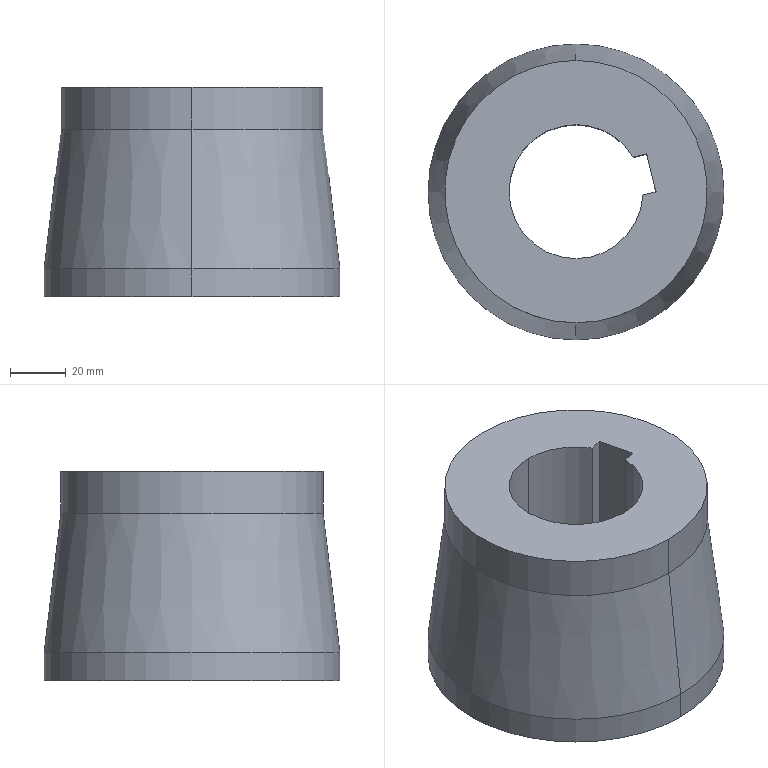Part | SolidWorks | features ICE 1, RevCut 1, Revolution 1 | 1 solid | 14 faces | box 106 x 106 x 75 mm | volume 445446 mm3 | cylinder 7 | plane 5 | cone 2 | commonest cylinder face diameters 48 x3 94 x2 106 x2
STEP:
#1=CARTESIAN_POINT('',(521.231,210.744,-1074.998));
#2=VERTEX_POINT('',#1);
#3=CARTESIAN_POINT('',(521.231,258.744,-1074.998));
#4=VERTEX_POINT('',#3);
#5=CARTESIAN_POINT('',(521.231,234.744,-1074.998));
#6=DIRECTION('',(0.,0.,-1.));
#7=DIRECTION('',(0.,1.,0.));
#8=AXIS2_PLACEMENT_3D('',#5,#6,#7);
#9=CIRCLE('',#8,24.);
#10=EDGE_CURVE('',#2,#4,#9,.T.);
#11=ORIENTED_EDGE('',*,*,#10,.F.);
#12=CARTESIAN_POINT('',(521.231,210.744,-1149.998));
#13=VERTEX_POINT('',#12);
#14=CARTESIAN_POINT('',(521.231,210.744,-1074.998));
#15=DIRECTION('',(0.,0.,-1.));
#16=VECTOR('',#15,1000.);
#17=LINE('',#14,#16);
#18=EDGE_CURVE('',#2,#13,#17,.T.);
#19=ORIENTED_EDGE('',*,*,#18,.T.);
#20=CARTESIAN_POINT('',(521.231,258.744,-1149.998));
#21=VERTEX_POINT('',#20);
#22=CARTESIAN_POINT('',(521.231,234.744,-1149.998));
#23=DIRECTION('',(0.,0.,-1.));
#24=DIRECTION('',(0.,1.,0.));
#25=AXIS2_PLACEMENT_3D('',#22,#23,#24);
#26=CIRCLE('',#25,24.);
#27=EDGE_CURVE('',#13,#21,#26,.T.);
#28=ORIENTED_EDGE('',*,*,#27,.T.);
#29=CARTESIAN_POINT('',(521.231,258.744,-1074.998));
#30=DIRECTION('',(0.,0.,-1.));
#31=VECTOR('',#30,1000.);
#32=LINE('',#29,#31);
#33=EDGE_CURVE('',#4,#21,#32,.T.);
#34=ORIENTED_EDGE('',*,*,#33,.F.);
#35=EDGE_LOOP('',(#11,#19,#28,#34));
#36=FACE_OUTER_BOUND('',#35,.T.);
#37=CARTESIAN_POINT('',(521.231,234.744,-1074.998));
#38=DIRECTION('',(0.,0.,-1.));
#39=DIRECTION('',(0.,1.,0.));
#40=AXIS2_PLACEMENT_3D('',#37,#38,#39);
#41=CYLINDRICAL_SURFACE('',#40,24.);
#42=ADVANCED_FACE('',(#36),#41,.F.);
#43=CARTESIAN_POINT('',(541.805,247.101,-1074.998));
#44=VERTEX_POINT('',#43);
#45=CARTESIAN_POINT('',(521.231,234.744,-1074.998));
#46=DIRECTION('',(0.,0.,-1.));
#47=DIRECTION('',(0.,1.,0.));
#48=AXIS2_PLACEMENT_3D('',#45,#46,#47);
#49=CIRCLE('',#48,24.);
#50=EDGE_CURVE('',#4,#44,#49,.T.);
#51=ORIENTED_EDGE('',*,*,#50,.F.);
#52=ORIENTED_EDGE('',*,*,#33,.T.);
#53=CARTESIAN_POINT('',(541.805,247.101,-1149.998));
#54=VERTEX_POINT('',#53);
#55=CARTESIAN_POINT('',(521.231,234.744,-1149.998));
#56=DIRECTION('',(0.,0.,-1.));
#57=DIRECTION('',(0.,1.,0.));
#58=AXIS2_PLACEMENT_3D('',#55,#56,#57);
#59=CIRCLE('',#58,24.);
#60=EDGE_CURVE('',#21,#54,#59,.T.);
#61=ORIENTED_EDGE('',*,*,#60,.T.);
#62=CARTESIAN_POINT('',(541.805,247.101,-1149.998));
#63=DIRECTION('',(0.,0.,1.));
#64=VECTOR('',#63,1000.);
#65=LINE('',#62,#64);
#66=EDGE_CURVE('',#54,#44,#65,.T.);
#67=ORIENTED_EDGE('',*,*,#66,.T.);
#68=EDGE_LOOP('',(#51,#52,#61,#67));
#69=FACE_OUTER_BOUND('',#68,.T.);
#70=CARTESIAN_POINT('',(521.231,234.744,-1074.998));
#71=DIRECTION('',(0.,0.,-1.));
#72=DIRECTION('',(0.,1.,0.));
#73=AXIS2_PLACEMENT_3D('',#70,#71,#72);
#74=CYLINDRICAL_SURFACE('',#73,24.);
#75=ADVANCED_FACE('',(#69),#74,.F.);
#76=CARTESIAN_POINT('',(521.231,287.744,-1139.998));
#77=VERTEX_POINT('',#76);
#78=CARTESIAN_POINT('',(521.231,181.744,-1139.998));
#79=VERTEX_POINT('',#78);
#80=CARTESIAN_POINT('',(521.231,234.744,-1139.998));
#81=DIRECTION('',(0.,0.,-1.));
#82=DIRECTION('',(0.,1.,0.));
#83=AXIS2_PLACEMENT_3D('',#80,#81,#82);
#84=CIRCLE('',#83,53.);
#85=EDGE_CURVE('',#77,#79,#84,.T.);
#86=ORIENTED_EDGE('',*,*,#85,.T.);
#87=CARTESIAN_POINT('',(521.231,181.744,-1149.998));
#88=VERTEX_POINT('',#87);
#89=CARTESIAN_POINT('',(521.231,181.744,-1074.998));
#90=DIRECTION('',(0.,0.,-1.));
#91=VECTOR('',#90,1000.);
#92=LINE('',#89,#91);
#93=EDGE_CURVE('',#79,#88,#92,.T.);
#94=ORIENTED_EDGE('',*,*,#93,.T.);
#95=CARTESIAN_POINT('',(521.231,287.744,-1149.998));
#96=VERTEX_POINT('',#95);
#97=CARTESIAN_POINT('',(521.231,234.744,-1149.998));
#98=DIRECTION('',(0.,0.,-1.));
#99=DIRECTION('',(0.,1.,0.));
#100=AXIS2_PLACEMENT_3D('',#97,#98,#99);
#101=CIRCLE('',#100,53.);
#102=EDGE_CURVE('',#96,#88,#101,.T.);
#103=ORIENTED_EDGE('',*,*,#102,.F.);
#104=CARTESIAN_POINT('',(521.231,287.744,-1074.998));
#105=DIRECTION('',(0.,0.,-1.));
#106=VECTOR('',#105,1000.);
#107=LINE('',#104,#106);
#108=EDGE_CURVE('',#77,#96,#107,.T.);
#109=ORIENTED_EDGE('',*,*,#108,.F.);
#110=EDGE_LOOP('',(#86,#94,#103,#109));
#111=FACE_OUTER_BOUND('',#110,.T.);
#112=CARTESIAN_POINT('',(521.231,234.744,-1074.998));
#113=DIRECTION('',(0.,0.,-1.));
#114=DIRECTION('',(0.,1.,0.));
#115=AXIS2_PLACEMENT_3D('',#112,#113,#114);
#116=CYLINDRICAL_SURFACE('',#115,53.);
#117=ADVANCED_FACE('',(#111),#116,.T.);
#118=CARTESIAN_POINT('',(521.231,281.744,-1089.998));
#119=VERTEX_POINT('',#118);
#120=CARTESIAN_POINT('',(521.231,187.744,-1089.998));
#121=VERTEX_POINT('',#120);
#122=CARTESIAN_POINT('',(521.231,234.744,-1089.998));
#123=DIRECTION('',(0.,0.,-1.));
#124=DIRECTION('',(0.,1.,0.));
#125=AXIS2_PLACEMENT_3D('',#122,#123,#124);
#126=CIRCLE('',#125,47.);
#127=EDGE_CURVE('',#119,#121,#126,.T.);
#128=ORIENTED_EDGE('',*,*,#127,.T.);
#129=CARTESIAN_POINT('',(521.231,181.744,-1139.998));
#130=DIRECTION('',(0.,-0.1191,-0.9929));
#131=VECTOR('',#130,1000.);
#132=LINE('',#129,#131);
#133=EDGE_CURVE('',#121,#79,#132,.T.);
#134=ORIENTED_EDGE('',*,*,#133,.T.);
#135=ORIENTED_EDGE('',*,*,#85,.F.);
#136=CARTESIAN_POINT('',(521.231,287.744,-1139.998));
#137=DIRECTION('',(0.,0.1191,-0.9929));
#138=VECTOR('',#137,1000.);
#139=LINE('',#136,#138);
#140=EDGE_CURVE('',#119,#77,#139,.T.);
#141=ORIENTED_EDGE('',*,*,#140,.F.);
#142=EDGE_LOOP('',(#128,#134,#135,#141));
#143=FACE_OUTER_BOUND('',#142,.T.);
#144=CARTESIAN_POINT('',(521.231,234.744,-1139.998));
#145=DIRECTION('',(0.,0.,-1.));
#146=DIRECTION('',(0.,1.,0.));
#147=AXIS2_PLACEMENT_3D('',#144,#145,#146);
#148=CONICAL_SURFACE('',#147,53.,0.1194);
#149=ADVANCED_FACE('',(#143),#148,.T.);
#150=CARTESIAN_POINT('',(521.231,281.744,-1074.998));
#151=VERTEX_POINT('',#150);
#152=CARTESIAN_POINT('',(521.231,187.744,-1074.998));
#153=VERTEX_POINT('',#152);
#154=CARTESIAN_POINT('',(521.231,234.744,-1074.998));
#155=DIRECTION('',(0.,0.,-1.));
#156=DIRECTION('',(0.,1.,0.));
#157=AXIS2_PLACEMENT_3D('',#154,#155,#156);
#158=CIRCLE('',#157,47.);
#159=EDGE_CURVE('',#151,#153,#158,.T.);
#160=ORIENTED_EDGE('',*,*,#159,.T.);
#161=CARTESIAN_POINT('',(521.231,187.744,-1074.998));
#162=DIRECTION('',(0.,0.,-1.));
#163=VECTOR('',#162,1000.);
#164=LINE('',#161,#163);
#165=EDGE_CURVE('',#153,#121,#164,.T.);
#166=ORIENTED_EDGE('',*,*,#165,.T.);
#167=ORIENTED_EDGE('',*,*,#127,.F.);
#168=CARTESIAN_POINT('',(521.231,281.744,-1074.998));
#169=DIRECTION('',(0.,0.,-1.));
#170=VECTOR('',#169,1000.);
#171=LINE('',#168,#170);
#172=EDGE_CURVE('',#151,#119,#171,.T.);
#173=ORIENTED_EDGE('',*,*,#172,.F.);
#174=EDGE_LOOP('',(#160,#166,#167,#173));
#175=FACE_OUTER_BOUND('',#174,.T.);
#176=CARTESIAN_POINT('',(521.231,234.744,-1074.998));
#177=DIRECTION('',(0.,0.,-1.));
#178=DIRECTION('',(0.,1.,0.));
#179=AXIS2_PLACEMENT_3D('',#176,#177,#178);
#180=CYLINDRICAL_SURFACE('',#179,47.);
#181=ADVANCED_FACE('',(#175),#180,.T.);
#182=ORIENTED_EDGE('',*,*,#165,.F.);
#183=CARTESIAN_POINT('',(521.231,234.744,-1074.998));
#184=DIRECTION('',(0.,0.,-1.));
#185=DIRECTION('',(0.,1.,0.));
#186=AXIS2_PLACEMENT_3D('',#183,#184,#185);
#187=CIRCLE('',#186,47.);
#188=EDGE_CURVE('',#153,#151,#187,.T.);
#189=ORIENTED_EDGE('',*,*,#188,.T.);
#190=ORIENTED_EDGE('',*,*,#172,.T.);
#191=CARTESIAN_POINT('',(521.231,234.744,-1089.998));
#192=DIRECTION('',(0.,0.,-1.));
#193=DIRECTION('',(0.,1.,0.));
#194=AXIS2_PLACEMENT_3D('',#191,#192,#193);
#195=CIRCLE('',#194,47.);
#196=EDGE_CURVE('',#121,#119,#195,.T.);
#197=ORIENTED_EDGE('',*,*,#196,.F.);
#198=EDGE_LOOP('',(#182,#189,#190,#197));
#199=FACE_OUTER_BOUND('',#198,.T.);
#200=CARTESIAN_POINT('',(521.231,234.744,-1074.998));
#201=DIRECTION('',(0.,0.,-1.));
#202=DIRECTION('',(0.,1.,0.));
#203=AXIS2_PLACEMENT_3D('',#200,#201,#202);
#204=CYLINDRICAL_SURFACE('',#203,47.);
#205=ADVANCED_FACE('',(#199),#204,.T.);
#206=ORIENTED_EDGE('',*,*,#133,.F.);
#207=ORIENTED_EDGE('',*,*,#196,.T.);
#208=ORIENTED_EDGE('',*,*,#140,.T.);
#209=CARTESIAN_POINT('',(521.231,234.744,-1139.998));
#210=DIRECTION('',(0.,0.,-1.));
#211=DIRECTION('',(0.,1.,0.));
#212=AXIS2_PLACEMENT_3D('',#209,#210,#211);
#213=CIRCLE('',#212,53.);
#214=EDGE_CURVE('',#79,#77,#213,.T.);
#215=ORIENTED_EDGE('',*,*,#214,.F.);
#216=EDGE_LOOP('',(#206,#207,#208,#215));
#217=FACE_OUTER_BOUND('',#216,.T.);
#218=CARTESIAN_POINT('',(521.231,234.744,-1139.998));
#219=DIRECTION('',(0.,0.,-1.));
#220=DIRECTION('',(0.,1.,0.));
#221=AXIS2_PLACEMENT_3D('',#218,#219,#220);
#222=CONICAL_SURFACE('',#221,53.,0.1194);
#223=ADVANCED_FACE('',(#217),#222,.T.);
#224=ORIENTED_EDGE('',*,*,#93,.F.);
#225=ORIENTED_EDGE('',*,*,#214,.T.);
#226=ORIENTED_EDGE('',*,*,#108,.T.);
#227=CARTESIAN_POINT('',(521.231,234.744,-1149.998));
#228=DIRECTION('',(0.,0.,-1.));
#229=DIRECTION('',(0.,1.,0.));
#230=AXIS2_PLACEMENT_3D('',#227,#228,#229);
#231=CIRCLE('',#230,53.);
#232=EDGE_CURVE('',#88,#96,#231,.T.);
#233=ORIENTED_EDGE('',*,*,#232,.F.);
#234=EDGE_LOOP('',(#224,#225,#226,#233));
#235=FACE_OUTER_BOUND('',#234,.T.);
#236=CARTESIAN_POINT('',(521.231,234.744,-1074.998));
#237=DIRECTION('',(0.,0.,-1.));
#238=DIRECTION('',(0.,1.,0.));
#239=AXIS2_PLACEMENT_3D('',#236,#237,#238);
#240=CYLINDRICAL_SURFACE('',#239,53.);
#241=ADVANCED_FACE('',(#235),#240,.T.);
#242=CARTESIAN_POINT('',(545.199,233.519,-1149.998));
#243=VERTEX_POINT('',#242);
#244=CARTESIAN_POINT('',(521.231,234.744,-1149.998));
#245=DIRECTION('',(0.,0.,-1.));
#246=DIRECTION('',(0.,1.,0.));
#247=AXIS2_PLACEMENT_3D('',#244,#245,#246);
#248=CIRCLE('',#247,24.);
#249=EDGE_CURVE('',#243,#13,#248,.T.);
#250=ORIENTED_EDGE('',*,*,#249,.F.);
#251=CARTESIAN_POINT('',(549.898,234.693,-1149.998));
#252=VERTEX_POINT('',#251);
#253=CARTESIAN_POINT('',(545.199,233.519,-1149.998));
#254=DIRECTION('',(0.9702,0.2424,0.));
#255=VECTOR('',#254,1000.);
#256=LINE('',#253,#255);
#257=EDGE_CURVE('',#243,#252,#256,.T.);
#258=ORIENTED_EDGE('',*,*,#257,.T.);
#259=CARTESIAN_POINT('',(546.504,248.275,-1149.998));
#260=VERTEX_POINT('',#259);
#261=CARTESIAN_POINT('',(549.898,234.693,-1149.998));
#262=DIRECTION('',(-0.2424,0.9702,0.));
#263=VECTOR('',#262,1000.);
#264=LINE('',#261,#263);
#265=EDGE_CURVE('',#252,#260,#264,.T.);
#266=ORIENTED_EDGE('',*,*,#265,.T.);
#267=CARTESIAN_POINT('',(546.504,248.275,-1149.998));
#268=DIRECTION('',(-0.9702,-0.2424,0.));
#269=VECTOR('',#268,1000.);
#270=LINE('',#267,#269);
#271=EDGE_CURVE('',#260,#54,#270,.T.);
#272=ORIENTED_EDGE('',*,*,#271,.T.);
#273=ORIENTED_EDGE('',*,*,#60,.F.);
#274=ORIENTED_EDGE('',*,*,#27,.F.);
#275=EDGE_LOOP('',(#250,#258,#266,#272,#273,#274));
#276=FACE_BOUND('',#275,.T.);
#277=ORIENTED_EDGE('',*,*,#102,.T.);
#278=ORIENTED_EDGE('',*,*,#232,.T.);
#279=EDGE_LOOP('',(#277,#278));
#280=FACE_OUTER_BOUND('',#279,.T.);
#281=CARTESIAN_POINT('',(521.231,234.744,-1149.998));
#282=DIRECTION('',(0.,0.,-1.));
#283=DIRECTION('',(0.,1.,0.));
#284=AXIS2_PLACEMENT_3D('',#281,#282,#283);
#285=PLANE('',#284);
#286=ADVANCED_FACE('',(#276,#280),#285,.T.);
#287=CARTESIAN_POINT('',(545.199,233.519,-1074.998));
#288=VERTEX_POINT('',#287);
#289=CARTESIAN_POINT('',(521.231,234.744,-1074.998));
#290=DIRECTION('',(0.,0.,-1.));
#291=DIRECTION('',(0.,1.,0.));
#292=AXIS2_PLACEMENT_3D('',#289,#290,#291);
#293=CIRCLE('',#292,24.);
#294=EDGE_CURVE('',#288,#2,#293,.T.);
#295=ORIENTED_EDGE('',*,*,#294,.T.);
#296=ORIENTED_EDGE('',*,*,#10,.T.);
#297=ORIENTED_EDGE('',*,*,#50,.T.);
#298=CARTESIAN_POINT('',(546.504,248.275,-1074.998));
#299=VERTEX_POINT('',#298);
#300=CARTESIAN_POINT('',(546.504,248.275,-1074.998));
#301=DIRECTION('',(-0.9702,-0.2424,0.));
#302=VECTOR('',#301,1000.);
#303=LINE('',#300,#302);
#304=EDGE_CURVE('',#299,#44,#303,.T.);
#305=ORIENTED_EDGE('',*,*,#304,.F.);
#306=CARTESIAN_POINT('',(549.898,234.693,-1074.998));
#307=VERTEX_POINT('',#306);
#308=CARTESIAN_POINT('',(549.898,234.693,-1074.998));
#309=DIRECTION('',(-0.2424,0.9702,0.));
#310=VECTOR('',#309,1000.);
#311=LINE('',#308,#310);
#312=EDGE_CURVE('',#307,#299,#311,.T.);
#313=ORIENTED_EDGE('',*,*,#312,.F.);
#314=CARTESIAN_POINT('',(545.199,233.519,-1074.998));
#315=DIRECTION('',(0.9702,0.2424,0.));
#316=VECTOR('',#315,1000.);
#317=LINE('',#314,#316);
#318=EDGE_CURVE('',#288,#307,#317,.T.);
#319=ORIENTED_EDGE('',*,*,#318,.F.);
#320=EDGE_LOOP('',(#295,#296,#297,#305,#313,#319));
#321=FACE_BOUND('',#320,.T.);
#322=ORIENTED_EDGE('',*,*,#159,.F.);
#323=ORIENTED_EDGE('',*,*,#188,.F.);
#324=EDGE_LOOP('',(#322,#323));
#325=FACE_OUTER_BOUND('',#324,.T.);
#326=CARTESIAN_POINT('',(568.231,234.744,-1074.998));
#327=DIRECTION('',(0.,0.,1.));
#328=DIRECTION('',(0.,-1.,0.));
#329=AXIS2_PLACEMENT_3D('',#326,#327,#328);
#330=PLANE('',#329);
#331=ADVANCED_FACE('',(#321,#325),#330,.T.);
#332=ORIENTED_EDGE('',*,*,#318,.T.);
#333=CARTESIAN_POINT('',(549.898,234.693,-1149.998));
#334=DIRECTION('',(0.,0.,1.));
#335=VECTOR('',#334,1000.);
#336=LINE('',#333,#335);
#337=EDGE_CURVE('',#252,#307,#336,.T.);
#338=ORIENTED_EDGE('',*,*,#337,.F.);
#339=ORIENTED_EDGE('',*,*,#257,.F.);
#340=CARTESIAN_POINT('',(545.199,233.519,-1149.998));
#341=DIRECTION('',(0.,0.,1.));
#342=VECTOR('',#341,1000.);
#343=LINE('',#340,#342);
#344=EDGE_CURVE('',#243,#288,#343,.T.);
#345=ORIENTED_EDGE('',*,*,#344,.T.);
#346=EDGE_LOOP('',(#332,#338,#339,#345));
#347=FACE_OUTER_BOUND('',#346,.T.);
#348=CARTESIAN_POINT('',(545.199,233.519,-1149.998));
#349=DIRECTION('',(0.2424,-0.9702,0.));
#350=DIRECTION('',(0.9702,0.2424,0.));
#351=AXIS2_PLACEMENT_3D('',#348,#349,#350);
#352=PLANE('',#351);
#353=ADVANCED_FACE('',(#347),#352,.F.);
#354=ORIENTED_EDGE('',*,*,#304,.T.);
#355=ORIENTED_EDGE('',*,*,#66,.F.);
#356=ORIENTED_EDGE('',*,*,#271,.F.);
#357=CARTESIAN_POINT('',(546.504,248.275,-1149.998));
#358=DIRECTION('',(0.,0.,1.));
#359=VECTOR('',#358,1000.);
#360=LINE('',#357,#359);
#361=EDGE_CURVE('',#260,#299,#360,.T.);
#362=ORIENTED_EDGE('',*,*,#361,.T.);
#363=EDGE_LOOP('',(#354,#355,#356,#362));
#364=FACE_OUTER_BOUND('',#363,.T.);
#365=CARTESIAN_POINT('',(546.504,248.275,-1149.998));
#366=DIRECTION('',(-0.2424,0.9702,0.));
#367=DIRECTION('',(-0.9702,-0.2424,0.));
#368=AXIS2_PLACEMENT_3D('',#365,#366,#367);
#369=PLANE('',#368);
#370=ADVANCED_FACE('',(#364),#369,.F.);
#371=ORIENTED_EDGE('',*,*,#312,.T.);
#372=ORIENTED_EDGE('',*,*,#361,.F.);
#373=ORIENTED_EDGE('',*,*,#265,.F.);
#374=ORIENTED_EDGE('',*,*,#337,.T.);
#375=EDGE_LOOP('',(#371,#372,#373,#374));
#376=FACE_OUTER_BOUND('',#375,.T.);
#377=CARTESIAN_POINT('',(549.898,234.693,-1149.998));
#378=DIRECTION('',(0.9702,0.2424,0.));
#379=DIRECTION('',(-0.2424,0.9702,0.));
#380=AXIS2_PLACEMENT_3D('',#377,#378,#379);
#381=PLANE('',#380);
#382=ADVANCED_FACE('',(#376),#381,.F.);
#383=ORIENTED_EDGE('',*,*,#18,.F.);
#384=ORIENTED_EDGE('',*,*,#294,.F.);
#385=ORIENTED_EDGE('',*,*,#344,.F.);
#386=ORIENTED_EDGE('',*,*,#249,.T.);
#387=EDGE_LOOP('',(#383,#384,#385,#386));
#388=FACE_OUTER_BOUND('',#387,.T.);
#389=CARTESIAN_POINT('',(521.231,234.744,-1074.998));
#390=DIRECTION('',(0.,0.,-1.));
#391=DIRECTION('',(0.,1.,0.));
#392=AXIS2_PLACEMENT_3D('',#389,#390,#391);
#393=CYLINDRICAL_SURFACE('',#392,24.);
#394=ADVANCED_FACE('',(#388),#393,.F.);
#395=CLOSED_SHELL('',(#42,#75,#117,#149,#181,#205,#223,#241,#286,#331,#353,#370,#382,#394));
#396=MANIFOLD_SOLID_BREP('',#395);
#397=CARTESIAN_POINT('',(0.,0.,0.));
#398=DIRECTION('',(0.,0.,1.));
#399=DIRECTION('',(1.,0.,0.));
#400=AXIS2_PLACEMENT_3D('',#397,#398,#399);
#401=(LENGTH_UNIT()NAMED_UNIT(*)SI_UNIT(.MILLI.,.METRE.));
#402=UNCERTAINTY_MEASURE_WITH_UNIT(LENGTH_MEASURE(0.00001),#401,'','');
#403=(NAMED_UNIT(*)PLANE_ANGLE_UNIT()SI_UNIT($,.RADIAN.));
#404=(NAMED_UNIT(*)SI_UNIT($,.STERADIAN.)SOLID_ANGLE_UNIT());
#405=(GEOMETRIC_REPRESENTATION_CONTEXT(3)GLOBAL_UNCERTAINTY_ASSIGNED_CONTEXT((#402))GLOBAL_UNIT_ASSIGNED_CONTEXT((#401,#403,#404))REPRESENTATION_CONTEXT('',''));
#406=ADVANCED_BREP_SHAPE_REPRESENTATION('',(#396,#400),#405);